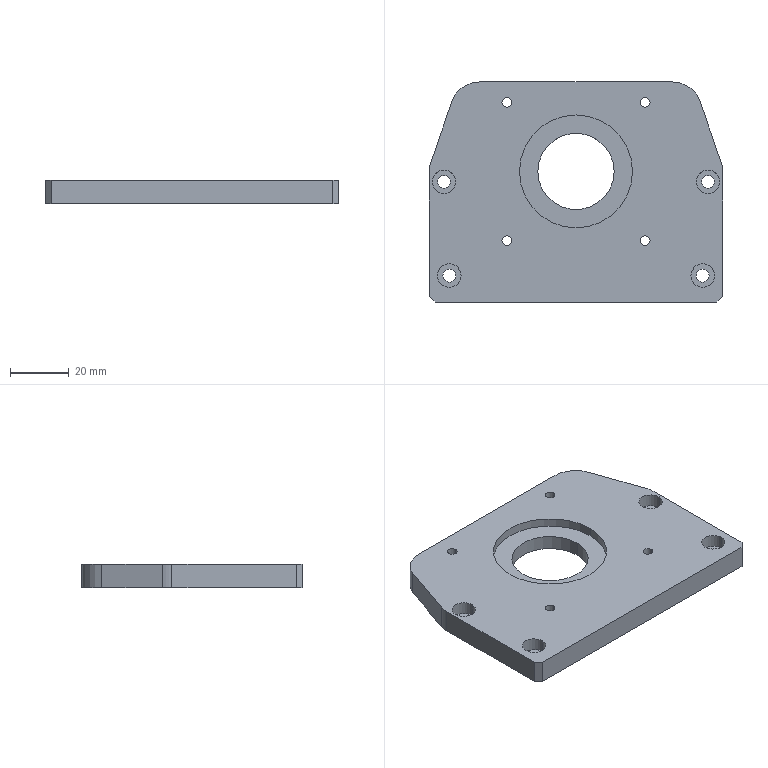Part | SolidWorks | features Cut 2, HoleWzd 2, Chamfer 1, Extrusion 1, Fillet 1, ICE 1 | 1 solid | 47 faces | box 100 x 75 x 8 mm | volume 49957 mm3 | cylinder 32 | plane 15 | commonest cylinder face diameters 3.3 x8 4.4 x8 8 x8 20 x4 26 x2 38.5 x2
STEP:
#1=CARTESIAN_POINT('',(-25.22,-16.57,0.));
#2=VERTEX_POINT('',#1);
#3=CARTESIAN_POINT('',(-21.92,-16.57,0.));
#4=VERTEX_POINT('',#3);
#5=CARTESIAN_POINT('',(-23.57,-16.57,0.));
#6=DIRECTION('',(0.,0.,1.));
#7=DIRECTION('',(1.,0.,0.));
#8=AXIS2_PLACEMENT_3D('',#5,#6,#7);
#9=CIRCLE('',#8,1.65);
#10=EDGE_CURVE('',#2,#4,#9,.T.);
#11=ORIENTED_EDGE('',*,*,#10,.F.);
#12=CARTESIAN_POINT('',(-25.22,-16.57,8.));
#13=VERTEX_POINT('',#12);
#14=CARTESIAN_POINT('',(-25.22,-16.57,8.));
#15=DIRECTION('',(0.,0.,1.));
#16=VECTOR('',#15,1000.);
#17=LINE('',#14,#16);
#18=EDGE_CURVE('',#2,#13,#17,.T.);
#19=ORIENTED_EDGE('',*,*,#18,.T.);
#20=CARTESIAN_POINT('',(-21.92,-16.57,8.));
#21=VERTEX_POINT('',#20);
#22=CARTESIAN_POINT('',(-23.57,-16.57,8.));
#23=DIRECTION('',(0.,0.,1.));
#24=DIRECTION('',(1.,0.,0.));
#25=AXIS2_PLACEMENT_3D('',#22,#23,#24);
#26=CIRCLE('',#25,1.65);
#27=EDGE_CURVE('',#13,#21,#26,.T.);
#28=ORIENTED_EDGE('',*,*,#27,.T.);
#29=CARTESIAN_POINT('',(-21.92,-16.57,8.));
#30=DIRECTION('',(0.,0.,1.));
#31=VECTOR('',#30,1000.);
#32=LINE('',#29,#31);
#33=EDGE_CURVE('',#4,#21,#32,.T.);
#34=ORIENTED_EDGE('',*,*,#33,.F.);
#35=EDGE_LOOP('',(#11,#19,#28,#34));
#36=FACE_OUTER_BOUND('',#35,.T.);
#37=CARTESIAN_POINT('',(-23.57,-16.57,8.));
#38=DIRECTION('',(0.,0.,1.));
#39=DIRECTION('',(1.,0.,0.));
#40=AXIS2_PLACEMENT_3D('',#37,#38,#39);
#41=CYLINDRICAL_SURFACE('',#40,1.65);
#42=ADVANCED_FACE('',(#36),#41,.F.);
#43=CARTESIAN_POINT('',(21.92,-16.57,0.));
#44=VERTEX_POINT('',#43);
#45=CARTESIAN_POINT('',(25.22,-16.57,0.));
#46=VERTEX_POINT('',#45);
#47=CARTESIAN_POINT('',(23.57,-16.57,0.));
#48=DIRECTION('',(0.,0.,1.));
#49=DIRECTION('',(1.,0.,0.));
#50=AXIS2_PLACEMENT_3D('',#47,#48,#49);
#51=CIRCLE('',#50,1.65);
#52=EDGE_CURVE('',#44,#46,#51,.T.);
#53=ORIENTED_EDGE('',*,*,#52,.F.);
#54=CARTESIAN_POINT('',(21.92,-16.57,8.));
#55=VERTEX_POINT('',#54);
#56=CARTESIAN_POINT('',(21.92,-16.57,8.));
#57=DIRECTION('',(0.,0.,1.));
#58=VECTOR('',#57,1000.);
#59=LINE('',#56,#58);
#60=EDGE_CURVE('',#44,#55,#59,.T.);
#61=ORIENTED_EDGE('',*,*,#60,.T.);
#62=CARTESIAN_POINT('',(25.22,-16.57,8.));
#63=VERTEX_POINT('',#62);
#64=CARTESIAN_POINT('',(23.57,-16.57,8.));
#65=DIRECTION('',(0.,0.,1.));
#66=DIRECTION('',(1.,0.,0.));
#67=AXIS2_PLACEMENT_3D('',#64,#65,#66);
#68=CIRCLE('',#67,1.65);
#69=EDGE_CURVE('',#55,#63,#68,.T.);
#70=ORIENTED_EDGE('',*,*,#69,.T.);
#71=CARTESIAN_POINT('',(25.22,-16.57,8.));
#72=DIRECTION('',(0.,0.,1.));
#73=VECTOR('',#72,1000.);
#74=LINE('',#71,#73);
#75=EDGE_CURVE('',#46,#63,#74,.T.);
#76=ORIENTED_EDGE('',*,*,#75,.F.);
#77=EDGE_LOOP('',(#53,#61,#70,#76));
#78=FACE_OUTER_BOUND('',#77,.T.);
#79=CARTESIAN_POINT('',(23.57,-16.57,8.));
#80=DIRECTION('',(0.,0.,1.));
#81=DIRECTION('',(1.,0.,0.));
#82=AXIS2_PLACEMENT_3D('',#79,#80,#81);
#83=CYLINDRICAL_SURFACE('',#82,1.65);
#84=ADVANCED_FACE('',(#78),#83,.F.);
#85=CARTESIAN_POINT('',(21.92,30.57,0.));
#86=VERTEX_POINT('',#85);
#87=CARTESIAN_POINT('',(25.22,30.57,0.));
#88=VERTEX_POINT('',#87);
#89=CARTESIAN_POINT('',(23.57,30.57,0.));
#90=DIRECTION('',(0.,0.,1.));
#91=DIRECTION('',(1.,0.,0.));
#92=AXIS2_PLACEMENT_3D('',#89,#90,#91);
#93=CIRCLE('',#92,1.65);
#94=EDGE_CURVE('',#86,#88,#93,.T.);
#95=ORIENTED_EDGE('',*,*,#94,.F.);
#96=CARTESIAN_POINT('',(21.92,30.57,8.));
#97=VERTEX_POINT('',#96);
#98=CARTESIAN_POINT('',(21.92,30.57,8.));
#99=DIRECTION('',(0.,0.,1.));
#100=VECTOR('',#99,1000.);
#101=LINE('',#98,#100);
#102=EDGE_CURVE('',#86,#97,#101,.T.);
#103=ORIENTED_EDGE('',*,*,#102,.T.);
#104=CARTESIAN_POINT('',(25.22,30.57,8.));
#105=VERTEX_POINT('',#104);
#106=CARTESIAN_POINT('',(23.57,30.57,8.));
#107=DIRECTION('',(0.,0.,1.));
#108=DIRECTION('',(1.,0.,0.));
#109=AXIS2_PLACEMENT_3D('',#106,#107,#108);
#110=CIRCLE('',#109,1.65);
#111=EDGE_CURVE('',#97,#105,#110,.T.);
#112=ORIENTED_EDGE('',*,*,#111,.T.);
#113=CARTESIAN_POINT('',(25.22,30.57,8.));
#114=DIRECTION('',(0.,0.,1.));
#115=VECTOR('',#114,1000.);
#116=LINE('',#113,#115);
#117=EDGE_CURVE('',#88,#105,#116,.T.);
#118=ORIENTED_EDGE('',*,*,#117,.F.);
#119=EDGE_LOOP('',(#95,#103,#112,#118));
#120=FACE_OUTER_BOUND('',#119,.T.);
#121=CARTESIAN_POINT('',(23.57,30.57,8.));
#122=DIRECTION('',(0.,0.,1.));
#123=DIRECTION('',(1.,0.,0.));
#124=AXIS2_PLACEMENT_3D('',#121,#122,#123);
#125=CYLINDRICAL_SURFACE('',#124,1.65);
#126=ADVANCED_FACE('',(#120),#125,.F.);
#127=CARTESIAN_POINT('',(-25.22,30.57,0.));
#128=VERTEX_POINT('',#127);
#129=CARTESIAN_POINT('',(-21.92,30.57,0.));
#130=VERTEX_POINT('',#129);
#131=CARTESIAN_POINT('',(-23.57,30.57,0.));
#132=DIRECTION('',(0.,0.,1.));
#133=DIRECTION('',(1.,0.,0.));
#134=AXIS2_PLACEMENT_3D('',#131,#132,#133);
#135=CIRCLE('',#134,1.65);
#136=EDGE_CURVE('',#128,#130,#135,.T.);
#137=ORIENTED_EDGE('',*,*,#136,.F.);
#138=CARTESIAN_POINT('',(-25.22,30.57,8.));
#139=VERTEX_POINT('',#138);
#140=CARTESIAN_POINT('',(-25.22,30.57,8.));
#141=DIRECTION('',(0.,0.,1.));
#142=VECTOR('',#141,1000.);
#143=LINE('',#140,#142);
#144=EDGE_CURVE('',#128,#139,#143,.T.);
#145=ORIENTED_EDGE('',*,*,#144,.T.);
#146=CARTESIAN_POINT('',(-21.92,30.57,8.));
#147=VERTEX_POINT('',#146);
#148=CARTESIAN_POINT('',(-23.57,30.57,8.));
#149=DIRECTION('',(0.,0.,1.));
#150=DIRECTION('',(1.,0.,0.));
#151=AXIS2_PLACEMENT_3D('',#148,#149,#150);
#152=CIRCLE('',#151,1.65);
#153=EDGE_CURVE('',#139,#147,#152,.T.);
#154=ORIENTED_EDGE('',*,*,#153,.T.);
#155=CARTESIAN_POINT('',(-21.92,30.57,8.));
#156=DIRECTION('',(0.,0.,1.));
#157=VECTOR('',#156,1000.);
#158=LINE('',#155,#157);
#159=EDGE_CURVE('',#130,#147,#158,.T.);
#160=ORIENTED_EDGE('',*,*,#159,.F.);
#161=EDGE_LOOP('',(#137,#145,#154,#160));
#162=FACE_OUTER_BOUND('',#161,.T.);
#163=CARTESIAN_POINT('',(-23.57,30.57,8.));
#164=DIRECTION('',(0.,0.,1.));
#165=DIRECTION('',(1.,0.,0.));
#166=AXIS2_PLACEMENT_3D('',#163,#164,#165);
#167=CYLINDRICAL_SURFACE('',#166,1.65);
#168=ADVANCED_FACE('',(#162),#167,.F.);
#169=CARTESIAN_POINT('',(-49.,3.5,3.5));
#170=VERTEX_POINT('',#169);
#171=CARTESIAN_POINT('',(-41.,3.5,3.5));
#172=VERTEX_POINT('',#171);
#173=CARTESIAN_POINT('',(-45.,3.5,3.5));
#174=DIRECTION('',(0.,0.,1.));
#175=DIRECTION('',(1.,0.,0.));
#176=AXIS2_PLACEMENT_3D('',#173,#174,#175);
#177=CIRCLE('',#176,4.);
#178=EDGE_CURVE('',#170,#172,#177,.T.);
#179=ORIENTED_EDGE('',*,*,#178,.F.);
#180=CARTESIAN_POINT('',(-49.,3.5,8.));
#181=VERTEX_POINT('',#180);
#182=CARTESIAN_POINT('',(-49.,3.5,8.));
#183=DIRECTION('',(0.,0.,1.));
#184=VECTOR('',#183,1000.);
#185=LINE('',#182,#184);
#186=EDGE_CURVE('',#170,#181,#185,.T.);
#187=ORIENTED_EDGE('',*,*,#186,.T.);
#188=CARTESIAN_POINT('',(-41.,3.5,8.));
#189=VERTEX_POINT('',#188);
#190=CARTESIAN_POINT('',(-45.,3.5,8.));
#191=DIRECTION('',(0.,0.,1.));
#192=DIRECTION('',(1.,0.,0.));
#193=AXIS2_PLACEMENT_3D('',#190,#191,#192);
#194=CIRCLE('',#193,4.);
#195=EDGE_CURVE('',#181,#189,#194,.T.);
#196=ORIENTED_EDGE('',*,*,#195,.T.);
#197=CARTESIAN_POINT('',(-41.,3.5,8.));
#198=DIRECTION('',(0.,0.,1.));
#199=VECTOR('',#198,1000.);
#200=LINE('',#197,#199);
#201=EDGE_CURVE('',#172,#189,#200,.T.);
#202=ORIENTED_EDGE('',*,*,#201,.F.);
#203=EDGE_LOOP('',(#179,#187,#196,#202));
#204=FACE_OUTER_BOUND('',#203,.T.);
#205=CARTESIAN_POINT('',(-45.,3.5,8.));
#206=DIRECTION('',(0.,0.,1.));
#207=DIRECTION('',(1.,0.,0.));
#208=AXIS2_PLACEMENT_3D('',#205,#206,#207);
#209=CYLINDRICAL_SURFACE('',#208,4.);
#210=ADVANCED_FACE('',(#204),#209,.F.);
#211=CARTESIAN_POINT('',(-47.2,3.5,0.));
#212=VERTEX_POINT('',#211);
#213=CARTESIAN_POINT('',(-42.8,3.5,0.));
#214=VERTEX_POINT('',#213);
#215=CARTESIAN_POINT('',(-45.,3.5,0.));
#216=DIRECTION('',(0.,0.,1.));
#217=DIRECTION('',(1.,0.,0.));
#218=AXIS2_PLACEMENT_3D('',#215,#216,#217);
#219=CIRCLE('',#218,2.2);
#220=EDGE_CURVE('',#212,#214,#219,.T.);
#221=ORIENTED_EDGE('',*,*,#220,.F.);
#222=CARTESIAN_POINT('',(-47.2,3.5,3.5));
#223=VERTEX_POINT('',#222);
#224=CARTESIAN_POINT('',(-47.2,3.5,8.));
#225=DIRECTION('',(0.,0.,1.));
#226=VECTOR('',#225,1000.);
#227=LINE('',#224,#226);
#228=EDGE_CURVE('',#212,#223,#227,.T.);
#229=ORIENTED_EDGE('',*,*,#228,.T.);
#230=CARTESIAN_POINT('',(-42.8,3.5,3.5));
#231=VERTEX_POINT('',#230);
#232=CARTESIAN_POINT('',(-45.,3.5,3.5));
#233=DIRECTION('',(0.,0.,1.));
#234=DIRECTION('',(1.,0.,0.));
#235=AXIS2_PLACEMENT_3D('',#232,#233,#234);
#236=CIRCLE('',#235,2.2);
#237=EDGE_CURVE('',#223,#231,#236,.T.);
#238=ORIENTED_EDGE('',*,*,#237,.T.);
#239=CARTESIAN_POINT('',(-42.8,3.5,8.));
#240=DIRECTION('',(0.,0.,1.));
#241=VECTOR('',#240,1000.);
#242=LINE('',#239,#241);
#243=EDGE_CURVE('',#214,#231,#242,.T.);
#244=ORIENTED_EDGE('',*,*,#243,.F.);
#245=EDGE_LOOP('',(#221,#229,#238,#244));
#246=FACE_OUTER_BOUND('',#245,.T.);
#247=CARTESIAN_POINT('',(-45.,3.5,8.));
#248=DIRECTION('',(0.,0.,1.));
#249=DIRECTION('',(1.,0.,0.));
#250=AXIS2_PLACEMENT_3D('',#247,#248,#249);
#251=CYLINDRICAL_SURFACE('',#250,2.2);
#252=ADVANCED_FACE('',(#246),#251,.F.);
#253=CARTESIAN_POINT('',(-47.15,-28.5,3.5));
#254=VERTEX_POINT('',#253);
#255=CARTESIAN_POINT('',(-39.15,-28.5,3.5));
#256=VERTEX_POINT('',#255);
#257=CARTESIAN_POINT('',(-43.15,-28.5,3.5));
#258=DIRECTION('',(0.,0.,1.));
#259=DIRECTION('',(1.,0.,0.));
#260=AXIS2_PLACEMENT_3D('',#257,#258,#259);
#261=CIRCLE('',#260,4.);
#262=EDGE_CURVE('',#254,#256,#261,.T.);
#263=ORIENTED_EDGE('',*,*,#262,.F.);
#264=CARTESIAN_POINT('',(-47.15,-28.5,8.));
#265=VERTEX_POINT('',#264);
#266=CARTESIAN_POINT('',(-47.15,-28.5,8.));
#267=DIRECTION('',(0.,0.,1.));
#268=VECTOR('',#267,1000.);
#269=LINE('',#266,#268);
#270=EDGE_CURVE('',#254,#265,#269,.T.);
#271=ORIENTED_EDGE('',*,*,#270,.T.);
#272=CARTESIAN_POINT('',(-39.15,-28.5,8.));
#273=VERTEX_POINT('',#272);
#274=CARTESIAN_POINT('',(-43.15,-28.5,8.));
#275=DIRECTION('',(0.,0.,1.));
#276=DIRECTION('',(1.,0.,0.));
#277=AXIS2_PLACEMENT_3D('',#274,#275,#276);
#278=CIRCLE('',#277,4.);
#279=EDGE_CURVE('',#265,#273,#278,.T.);
#280=ORIENTED_EDGE('',*,*,#279,.T.);
#281=CARTESIAN_POINT('',(-39.15,-28.5,8.));
#282=DIRECTION('',(0.,0.,1.));
#283=VECTOR('',#282,1000.);
#284=LINE('',#281,#283);
#285=EDGE_CURVE('',#256,#273,#284,.T.);
#286=ORIENTED_EDGE('',*,*,#285,.F.);
#287=EDGE_LOOP('',(#263,#271,#280,#286));
#288=FACE_OUTER_BOUND('',#287,.T.);
#289=CARTESIAN_POINT('',(-43.15,-28.5,8.));
#290=DIRECTION('',(0.,0.,1.));
#291=DIRECTION('',(1.,0.,0.));
#292=AXIS2_PLACEMENT_3D('',#289,#290,#291);
#293=CYLINDRICAL_SURFACE('',#292,4.);
#294=ADVANCED_FACE('',(#288),#293,.F.);
#295=CARTESIAN_POINT('',(-45.35,-28.5,0.));
#296=VERTEX_POINT('',#295);
#297=CARTESIAN_POINT('',(-40.95,-28.5,0.));
#298=VERTEX_POINT('',#297);
#299=CARTESIAN_POINT('',(-43.15,-28.5,0.));
#300=DIRECTION('',(0.,0.,1.));
#301=DIRECTION('',(1.,0.,0.));
#302=AXIS2_PLACEMENT_3D('',#299,#300,#301);
#303=CIRCLE('',#302,2.2);
#304=EDGE_CURVE('',#296,#298,#303,.T.);
#305=ORIENTED_EDGE('',*,*,#304,.F.);
#306=CARTESIAN_POINT('',(-45.35,-28.5,3.5));
#307=VERTEX_POINT('',#306);
#308=CARTESIAN_POINT('',(-45.35,-28.5,8.));
#309=DIRECTION('',(0.,0.,1.));
#310=VECTOR('',#309,1000.);
#311=LINE('',#308,#310);
#312=EDGE_CURVE('',#296,#307,#311,.T.);
#313=ORIENTED_EDGE('',*,*,#312,.T.);
#314=CARTESIAN_POINT('',(-40.95,-28.5,3.5));
#315=VERTEX_POINT('',#314);
#316=CARTESIAN_POINT('',(-43.15,-28.5,3.5));
#317=DIRECTION('',(0.,0.,1.));
#318=DIRECTION('',(1.,0.,0.));
#319=AXIS2_PLACEMENT_3D('',#316,#317,#318);
#320=CIRCLE('',#319,2.2);
#321=EDGE_CURVE('',#307,#315,#320,.T.);
#322=ORIENTED_EDGE('',*,*,#321,.T.);
#323=CARTESIAN_POINT('',(-40.95,-28.5,8.));
#324=DIRECTION('',(0.,0.,1.));
#325=VECTOR('',#324,1000.);
#326=LINE('',#323,#325);
#327=EDGE_CURVE('',#298,#315,#326,.T.);
#328=ORIENTED_EDGE('',*,*,#327,.F.);
#329=EDGE_LOOP('',(#305,#313,#322,#328));
#330=FACE_OUTER_BOUND('',#329,.T.);
#331=CARTESIAN_POINT('',(-43.15,-28.5,8.));
#332=DIRECTION('',(0.,0.,1.));
#333=DIRECTION('',(1.,0.,0.));
#334=AXIS2_PLACEMENT_3D('',#331,#332,#333);
#335=CYLINDRICAL_SURFACE('',#334,2.2);
#336=ADVANCED_FACE('',(#330),#335,.F.);
#337=CARTESIAN_POINT('',(39.15,-28.5,3.5));
#338=VERTEX_POINT('',#337);
#339=CARTESIAN_POINT('',(47.15,-28.5,3.5));
#340=VERTEX_POINT('',#339);
#341=CARTESIAN_POINT('',(43.15,-28.5,3.5));
#342=DIRECTION('',(0.,0.,1.));
#343=DIRECTION('',(1.,0.,0.));
#344=AXIS2_PLACEMENT_3D('',#341,#342,#343);
#345=CIRCLE('',#344,4.);
#346=EDGE_CURVE('',#338,#340,#345,.T.);
#347=ORIENTED_EDGE('',*,*,#346,.F.);
#348=CARTESIAN_POINT('',(39.15,-28.5,8.));
#349=VERTEX_POINT('',#348);
#350=CARTESIAN_POINT('',(39.15,-28.5,8.));
#351=DIRECTION('',(0.,0.,1.));
#352=VECTOR('',#351,1000.);
#353=LINE('',#350,#352);
#354=EDGE_CURVE('',#338,#349,#353,.T.);
#355=ORIENTED_EDGE('',*,*,#354,.T.);
#356=CARTESIAN_POINT('',(47.15,-28.5,8.));
#357=VERTEX_POINT('',#356);
#358=CARTESIAN_POINT('',(43.15,-28.5,8.));
#359=DIRECTION('',(0.,0.,1.));
#360=DIRECTION('',(1.,0.,0.));
#361=AXIS2_PLACEMENT_3D('',#358,#359,#360);
#362=CIRCLE('',#361,4.);
#363=EDGE_CURVE('',#349,#357,#362,.T.);
#364=ORIENTED_EDGE('',*,*,#363,.T.);
#365=CARTESIAN_POINT('',(47.15,-28.5,8.));
#366=DIRECTION('',(0.,0.,1.));
#367=VECTOR('',#366,1000.);
#368=LINE('',#365,#367);
#369=EDGE_CURVE('',#340,#357,#368,.T.);
#370=ORIENTED_EDGE('',*,*,#369,.F.);
#371=EDGE_LOOP('',(#347,#355,#364,#370));
#372=FACE_OUTER_BOUND('',#371,.T.);
#373=CARTESIAN_POINT('',(43.15,-28.5,8.));
#374=DIRECTION('',(0.,0.,1.));
#375=DIRECTION('',(1.,0.,0.));
#376=AXIS2_PLACEMENT_3D('',#373,#374,#375);
#377=CYLINDRICAL_SURFACE('',#376,4.);
#378=ADVANCED_FACE('',(#372),#377,.F.);
#379=CARTESIAN_POINT('',(40.95,-28.5,0.));
#380=VERTEX_POINT('',#379);
#381=CARTESIAN_POINT('',(45.35,-28.5,0.));
#382=VERTEX_POINT('',#381);
#383=CARTESIAN_POINT('',(43.15,-28.5,0.));
#384=DIRECTION('',(0.,0.,1.));
#385=DIRECTION('',(1.,0.,0.));
#386=AXIS2_PLACEMENT_3D('',#383,#384,#385);
#387=CIRCLE('',#386,2.2);
#388=EDGE_CURVE('',#380,#382,#387,.T.);
#389=ORIENTED_EDGE('',*,*,#388,.F.);
#390=CARTESIAN_POINT('',(40.95,-28.5,3.5));
#391=VERTEX_POINT('',#390);
#392=CARTESIAN_POINT('',(40.95,-28.5,8.));
#393=DIRECTION('',(0.,0.,1.));
#394=VECTOR('',#393,1000.);
#395=LINE('',#392,#394);
#396=EDGE_CURVE('',#380,#391,#395,.T.);
#397=ORIENTED_EDGE('',*,*,#396,.T.);
#398=CARTESIAN_POINT('',(45.35,-28.5,3.5));
#399=VERTEX_POINT('',#398);
#400=CARTESIAN_POINT('',(43.15,-28.5,3.5));
#401=DIRECTION('',(0.,0.,1.));
#402=DIRECTION('',(1.,0.,0.));
#403=AXIS2_PLACEMENT_3D('',#400,#401,#402);
#404=CIRCLE('',#403,2.2);
#405=EDGE_CURVE('',#391,#399,#404,.T.);
#406=ORIENTED_EDGE('',*,*,#405,.T.);
#407=CARTESIAN_POINT('',(45.35,-28.5,8.));
#408=DIRECTION('',(0.,0.,1.));
#409=VECTOR('',#408,1000.);
#410=LINE('',#407,#409);
#411=EDGE_CURVE('',#382,#399,#410,.T.);
#412=ORIENTED_EDGE('',*,*,#411,.F.);
#413=EDGE_LOOP('',(#389,#397,#406,#412));
#414=FACE_OUTER_BOUND('',#413,.T.);
#415=CARTESIAN_POINT('',(43.15,-28.5,8.));
#416=DIRECTION('',(0.,0.,1.));
#417=DIRECTION('',(1.,0.,0.));
#418=AXIS2_PLACEMENT_3D('',#415,#416,#417);
#419=CYLINDRICAL_SURFACE('',#418,2.2);
#420=ADVANCED_FACE('',(#414),#419,.F.);
#421=CARTESIAN_POINT('',(41.,3.5,3.5));
#422=VERTEX_POINT('',#421);
#423=CARTESIAN_POINT('',(49.,3.5,3.5));
#424=VERTEX_POINT('',#423);
#425=CARTESIAN_POINT('',(45.,3.5,3.5));
#426=DIRECTION('',(0.,0.,1.));
#427=DIRECTION('',(1.,0.,0.));
#428=AXIS2_PLACEMENT_3D('',#425,#426,#427);
#429=CIRCLE('',#428,4.);
#430=EDGE_CURVE('',#422,#424,#429,.T.);
#431=ORIENTED_EDGE('',*,*,#430,.F.);
#432=CARTESIAN_POINT('',(41.,3.5,8.));
#433=VERTEX_POINT('',#432);
#434=CARTESIAN_POINT('',(41.,3.5,8.));
#435=DIRECTION('',(0.,0.,1.));
#436=VECTOR('',#435,1000.);
#437=LINE('',#434,#436);
#438=EDGE_CURVE('',#422,#433,#437,.T.);
#439=ORIENTED_EDGE('',*,*,#438,.T.);
#440=CARTESIAN_POINT('',(49.,3.5,8.));
#441=VERTEX_POINT('',#440);
#442=CARTESIAN_POINT('',(45.,3.5,8.));
#443=DIRECTION('',(0.,0.,1.));
#444=DIRECTION('',(1.,0.,0.));
#445=AXIS2_PLACEMENT_3D('',#442,#443,#444);
#446=CIRCLE('',#445,4.);
#447=EDGE_CURVE('',#433,#441,#446,.T.);
#448=ORIENTED_EDGE('',*,*,#447,.T.);
#449=CARTESIAN_POINT('',(49.,3.5,8.));
#450=DIRECTION('',(0.,0.,1.));
#451=VECTOR('',#450,1000.);
#452=LINE('',#449,#451);
#453=EDGE_CURVE('',#424,#441,#452,.T.);
#454=ORIENTED_EDGE('',*,*,#453,.F.);
#455=EDGE_LOOP('',(#431,#439,#448,#454));
#456=FACE_OUTER_BOUND('',#455,.T.);
#457=CARTESIAN_POINT('',(45.,3.5,8.));
#458=DIRECTION('',(0.,0.,1.));
#459=DIRECTION('',(1.,0.,0.));
#460=AXIS2_PLACEMENT_3D('',#457,#458,#459);
#461=CYLINDRICAL_SURFACE('',#460,4.);
#462=ADVANCED_FACE('',(#456),#461,.F.);
#463=CARTESIAN_POINT('',(42.8,3.5,0.));
#464=VERTEX_POINT('',#463);
#465=CARTESIAN_POINT('',(47.2,3.5,0.));
#466=VERTEX_POINT('',#465);
#467=CARTESIAN_POINT('',(45.,3.5,0.));
#468=DIRECTION('',(0.,0.,1.));
#469=DIRECTION('',(1.,0.,0.));
#470=AXIS2_PLACEMENT_3D('',#467,#468,#469);
#471=CIRCLE('',#470,2.2);
#472=EDGE_CURVE('',#464,#466,#471,.T.);
#473=ORIENTED_EDGE('',*,*,#472,.F.);
#474=CARTESIAN_POINT('',(42.8,3.5,3.5));
#475=VERTEX_POINT('',#474);
#476=CARTESIAN_POINT('',(42.8,3.5,8.));
#477=DIRECTION('',(0.,0.,1.));
#478=VECTOR('',#477,1000.);
#479=LINE('',#476,#478);
#480=EDGE_CURVE('',#464,#475,#479,.T.);
#481=ORIENTED_EDGE('',*,*,#480,.T.);
#482=CARTESIAN_POINT('',(47.2,3.5,3.5));
#483=VERTEX_POINT('',#482);
#484=CARTESIAN_POINT('',(45.,3.5,3.5));
#485=DIRECTION('',(0.,0.,1.));
#486=DIRECTION('',(1.,0.,0.));
#487=AXIS2_PLACEMENT_3D('',#484,#485,#486);
#488=CIRCLE('',#487,2.2);
#489=EDGE_CURVE('',#475,#483,#488,.T.);
#490=ORIENTED_EDGE('',*,*,#489,.T.);
#491=CARTESIAN_POINT('',(47.2,3.5,8.));
#492=DIRECTION('',(0.,0.,1.));
#493=VECTOR('',#492,1000.);
#494=LINE('',#491,#493);
#495=EDGE_CURVE('',#466,#483,#494,.T.);
#496=ORIENTED_EDGE('',*,*,#495,.F.);
#497=EDGE_LOOP('',(#473,#481,#490,#496));
#498=FACE_OUTER_BOUND('',#497,.T.);
#499=CARTESIAN_POINT('',(45.,3.5,8.));
#500=DIRECTION('',(0.,0.,1.));
#501=DIRECTION('',(1.,0.,0.));
#502=AXIS2_PLACEMENT_3D('',#499,#500,#501);
#503=CYLINDRICAL_SURFACE('',#502,2.2);
#504=ADVANCED_FACE('',(#498),#503,.F.);
#505=CARTESIAN_POINT('',(-13.,7.,0.));
#506=VERTEX_POINT('',#505);
#507=CARTESIAN_POINT('',(13.,7.,0.));
#508=VERTEX_POINT('',#507);
#509=CARTESIAN_POINT('',(0.,7.,0.));
#510=DIRECTION('',(0.,0.,1.));
#511=DIRECTION('',(1.,0.,0.));
#512=AXIS2_PLACEMENT_3D('',#509,#510,#511);
#513=CIRCLE('',#512,13.);
#514=EDGE_CURVE('',#506,#508,#513,.T.);
#515=ORIENTED_EDGE('',*,*,#514,.F.);
#516=CARTESIAN_POINT('',(-13.,7.,5.));
#517=VERTEX_POINT('',#516);
#518=CARTESIAN_POINT('',(-13.,7.,0.));
#519=DIRECTION('',(0.,0.,1.));
#520=VECTOR('',#519,1000.);
#521=LINE('',#518,#520);
#522=EDGE_CURVE('',#506,#517,#521,.T.);
#523=ORIENTED_EDGE('',*,*,#522,.T.);
#524=CARTESIAN_POINT('',(13.,7.,5.));
#525=VERTEX_POINT('',#524);
#526=CARTESIAN_POINT('',(0.,7.,5.));
#527=DIRECTION('',(0.,0.,1.));
#528=DIRECTION('',(1.,0.,0.));
#529=AXIS2_PLACEMENT_3D('',#526,#527,#528);
#530=CIRCLE('',#529,13.);
#531=EDGE_CURVE('',#517,#525,#530,.T.);
#532=ORIENTED_EDGE('',*,*,#531,.T.);
#533=CARTESIAN_POINT('',(13.,7.,0.));
#534=DIRECTION('',(0.,0.,1.));
#535=VECTOR('',#534,1000.);
#536=LINE('',#533,#535);
#537=EDGE_CURVE('',#508,#525,#536,.T.);
#538=ORIENTED_EDGE('',*,*,#537,.F.);
#539=EDGE_LOOP('',(#515,#523,#532,#538));
#540=FACE_OUTER_BOUND('',#539,.T.);
#541=CARTESIAN_POINT('',(0.,7.,0.));
#542=DIRECTION('',(0.,0.,1.));
#543=DIRECTION('',(1.,0.,0.));
#544=AXIS2_PLACEMENT_3D('',#541,#542,#543);
#545=CYLINDRICAL_SURFACE('',#544,13.);
#546=ADVANCED_FACE('',(#540),#545,.F.);
#547=CARTESIAN_POINT('',(-19.25,7.,5.));
#548=VERTEX_POINT('',#547);
#549=CARTESIAN_POINT('',(19.25,7.,5.));
#550=VERTEX_POINT('',#549);
#551=CARTESIAN_POINT('',(0.,7.,5.));
#552=DIRECTION('',(0.,0.,1.));
#553=DIRECTION('',(1.,0.,0.));
#554=AXIS2_PLACEMENT_3D('',#551,#552,#553);
#555=CIRCLE('',#554,19.25);
#556=EDGE_CURVE('',#548,#550,#555,.T.);
#557=ORIENTED_EDGE('',*,*,#556,.F.);
#558=CARTESIAN_POINT('',(-19.25,7.,8.));
#559=VERTEX_POINT('',#558);
#560=CARTESIAN_POINT('',(-19.25,7.,5.));
#561=DIRECTION('',(0.,0.,1.));
#562=VECTOR('',#561,1000.);
#563=LINE('',#560,#562);
#564=EDGE_CURVE('',#548,#559,#563,.T.);
#565=ORIENTED_EDGE('',*,*,#564,.T.);
#566=CARTESIAN_POINT('',(19.25,7.,8.));
#567=VERTEX_POINT('',#566);
#568=CARTESIAN_POINT('',(0.,7.,8.));
#569=DIRECTION('',(0.,0.,1.));
#570=DIRECTION('',(1.,0.,0.));
#571=AXIS2_PLACEMENT_3D('',#568,#569,#570);
#572=CIRCLE('',#571,19.25);
#573=EDGE_CURVE('',#559,#567,#572,.T.);
#574=ORIENTED_EDGE('',*,*,#573,.T.);
#575=CARTESIAN_POINT('',(19.25,7.,5.));
#576=DIRECTION('',(0.,0.,1.));
#577=VECTOR('',#576,1000.);
#578=LINE('',#575,#577);
#579=EDGE_CURVE('',#550,#567,#578,.T.);
#580=ORIENTED_EDGE('',*,*,#579,.F.);
#581=EDGE_LOOP('',(#557,#565,#574,#580));
#582=FACE_OUTER_BOUND('',#581,.T.);
#583=CARTESIAN_POINT('',(0.,7.,5.));
#584=DIRECTION('',(0.,0.,1.));
#585=DIRECTION('',(1.,0.,0.));
#586=AXIS2_PLACEMENT_3D('',#583,#584,#585);
#587=CYLINDRICAL_SURFACE('',#586,19.25);
#588=ADVANCED_FACE('',(#582),#587,.F.);
#589=CARTESIAN_POINT('',(50.,-35.5,8.));
#590=VERTEX_POINT('',#589);
#591=CARTESIAN_POINT('',(50.,6.824,8.));
#592=VERTEX_POINT('',#591);
#593=CARTESIAN_POINT('',(50.,-37.5,8.));
#594=DIRECTION('',(0.,1.,0.));
#595=VECTOR('',#594,1000.);
#596=LINE('',#593,#595);
#597=EDGE_CURVE('',#590,#592,#596,.T.);
#598=ORIENTED_EDGE('',*,*,#597,.F.);
#599=CARTESIAN_POINT('',(50.,-35.5,0.));
#600=VERTEX_POINT('',#599);
#601=CARTESIAN_POINT('',(50.,-35.5,8.));
#602=DIRECTION('',(0.,0.,-1.));
#603=VECTOR('',#602,1000.);
#604=LINE('',#601,#603);
#605=EDGE_CURVE('',#590,#600,#604,.T.);
#606=ORIENTED_EDGE('',*,*,#605,.T.);
#607=CARTESIAN_POINT('',(50.,6.824,0.));
#608=VERTEX_POINT('',#607);
#609=CARTESIAN_POINT('',(50.,-37.5,0.));
#610=DIRECTION('',(0.,1.,0.));
#611=VECTOR('',#610,1000.);
#612=LINE('',#609,#611);
#613=EDGE_CURVE('',#600,#608,#612,.T.);
#614=ORIENTED_EDGE('',*,*,#613,.T.);
#615=CARTESIAN_POINT('',(50.,6.824,8.));
#616=DIRECTION('',(0.,0.,1.));
#617=VECTOR('',#616,1000.);
#618=LINE('',#615,#617);
#619=EDGE_CURVE('',#608,#592,#618,.T.);
#620=ORIENTED_EDGE('',*,*,#619,.T.);
#621=EDGE_LOOP('',(#598,#606,#614,#620));
#622=FACE_OUTER_BOUND('',#621,.T.);
#623=CARTESIAN_POINT('',(50.,-37.5,8.));
#624=DIRECTION('',(-1.,0.,0.));
#625=DIRECTION('',(0.,0.,1.));
#626=AXIS2_PLACEMENT_3D('',#623,#624,#625);
#627=PLANE('',#626);
#628=ADVANCED_FACE('',(#622),#627,.F.);
#629=CARTESIAN_POINT('',(32.87,37.5,0.));
#630=VERTEX_POINT('',#629);
#631=CARTESIAN_POINT('',(-32.87,37.5,0.));
#632=VERTEX_POINT('',#631);
#633=CARTESIAN_POINT('',(-50.,37.5,0.));
#634=DIRECTION('',(-1.,0.,0.));
#635=VECTOR('',#634,1000.);
#636=LINE('',#633,#635);
#637=EDGE_CURVE('',#630,#632,#636,.T.);
#638=ORIENTED_EDGE('',*,*,#637,.T.);
#639=CARTESIAN_POINT('',(-32.87,37.5,8.));
#640=VERTEX_POINT('',#639);
#641=CARTESIAN_POINT('',(-32.87,37.5,8.));
#642=DIRECTION('',(0.,0.,1.));
#643=VECTOR('',#642,1000.);
#644=LINE('',#641,#643);
#645=EDGE_CURVE('',#632,#640,#644,.T.);
#646=ORIENTED_EDGE('',*,*,#645,.T.);
#647=CARTESIAN_POINT('',(32.87,37.5,8.));
#648=VERTEX_POINT('',#647);
#649=CARTESIAN_POINT('',(-50.,37.5,8.));
#650=DIRECTION('',(-1.,0.,0.));
#651=VECTOR('',#650,1000.);
#652=LINE('',#649,#651);
#653=EDGE_CURVE('',#648,#640,#652,.T.);
#654=ORIENTED_EDGE('',*,*,#653,.F.);
#655=CARTESIAN_POINT('',(32.87,37.5,8.));
#656=DIRECTION('',(0.,0.,-1.));
#657=VECTOR('',#656,1000.);
#658=LINE('',#655,#657);
#659=EDGE_CURVE('',#648,#630,#658,.T.);
#660=ORIENTED_EDGE('',*,*,#659,.T.);
#661=EDGE_LOOP('',(#638,#646,#654,#660));
#662=FACE_OUTER_BOUND('',#661,.T.);
#663=CARTESIAN_POINT('',(-50.,37.5,8.));
#664=DIRECTION('',(0.,-1.,0.));
#665=DIRECTION('',(0.,0.,-1.));
#666=AXIS2_PLACEMENT_3D('',#663,#664,#665);
#667=PLANE('',#666);
#668=ADVANCED_FACE('',(#662),#667,.F.);
#669=CARTESIAN_POINT('',(-50.,6.824,0.));
#670=VERTEX_POINT('',#669);
#671=CARTESIAN_POINT('',(-50.,-35.5,0.));
#672=VERTEX_POINT('',#671);
#673=CARTESIAN_POINT('',(-50.,-37.5,0.));
#674=DIRECTION('',(0.,-1.,0.));
#675=VECTOR('',#674,1000.);
#676=LINE('',#673,#675);
#677=EDGE_CURVE('',#670,#672,#676,.T.);
#678=ORIENTED_EDGE('',*,*,#677,.T.);
#679=CARTESIAN_POINT('',(-50.,-35.5,8.));
#680=VERTEX_POINT('',#679);
#681=CARTESIAN_POINT('',(-50.,-35.5,8.));
#682=DIRECTION('',(0.,0.,1.));
#683=VECTOR('',#682,1000.);
#684=LINE('',#681,#683);
#685=EDGE_CURVE('',#672,#680,#684,.T.);
#686=ORIENTED_EDGE('',*,*,#685,.T.);
#687=CARTESIAN_POINT('',(-50.,6.824,8.));
#688=VERTEX_POINT('',#687);
#689=CARTESIAN_POINT('',(-50.,-37.5,8.));
#690=DIRECTION('',(0.,-1.,0.));
#691=VECTOR('',#690,1000.);
#692=LINE('',#689,#691);
#693=EDGE_CURVE('',#688,#680,#692,.T.);
#694=ORIENTED_EDGE('',*,*,#693,.F.);
#695=CARTESIAN_POINT('',(-50.,6.824,8.));
#696=DIRECTION('',(0.,0.,-1.));
#697=VECTOR('',#696,1000.);
#698=LINE('',#695,#697);
#699=EDGE_CURVE('',#688,#670,#698,.T.);
#700=ORIENTED_EDGE('',*,*,#699,.T.);
#701=EDGE_LOOP('',(#678,#686,#694,#700));
#702=FACE_OUTER_BOUND('',#701,.T.);
#703=CARTESIAN_POINT('',(-50.,-37.5,8.));
#704=DIRECTION('',(1.,0.,0.));
#705=DIRECTION('',(0.,0.,-1.));
#706=AXIS2_PLACEMENT_3D('',#703,#704,#705);
#707=PLANE('',#706);
#708=ADVANCED_FACE('',(#702),#707,.F.);
#709=CARTESIAN_POINT('',(-48.,-37.5,8.));
#710=VERTEX_POINT('',#709);
#711=CARTESIAN_POINT('',(48.,-37.5,8.));
#712=VERTEX_POINT('',#711);
#713=CARTESIAN_POINT('',(-50.,-37.5,8.));
#714=DIRECTION('',(1.,0.,0.));
#715=VECTOR('',#714,1000.);
#716=LINE('',#713,#715);
#717=EDGE_CURVE('',#710,#712,#716,.T.);
#718=ORIENTED_EDGE('',*,*,#717,.F.);
#719=CARTESIAN_POINT('',(-48.,-37.5,0.));
#720=VERTEX_POINT('',#719);
#721=CARTESIAN_POINT('',(-48.,-37.5,8.));
#722=DIRECTION('',(0.,0.,-1.));
#723=VECTOR('',#722,1000.);
#724=LINE('',#721,#723);
#725=EDGE_CURVE('',#710,#720,#724,.T.);
#726=ORIENTED_EDGE('',*,*,#725,.T.);
#727=CARTESIAN_POINT('',(48.,-37.5,0.));
#728=VERTEX_POINT('',#727);
#729=CARTESIAN_POINT('',(-50.,-37.5,0.));
#730=DIRECTION('',(1.,0.,0.));
#731=VECTOR('',#730,1000.);
#732=LINE('',#729,#731);
#733=EDGE_CURVE('',#720,#728,#732,.T.);
#734=ORIENTED_EDGE('',*,*,#733,.T.);
#735=CARTESIAN_POINT('',(48.,-37.5,8.));
#736=DIRECTION('',(0.,0.,1.));
#737=VECTOR('',#736,1000.);
#738=LINE('',#735,#737);
#739=EDGE_CURVE('',#728,#712,#738,.T.);
#740=ORIENTED_EDGE('',*,*,#739,.T.);
#741=EDGE_LOOP('',(#718,#726,#734,#740));
#742=FACE_OUTER_BOUND('',#741,.T.);
#743=CARTESIAN_POINT('',(-50.,-37.5,8.));
#744=DIRECTION('',(0.,1.,0.));
#745=DIRECTION('',(0.,0.,1.));
#746=AXIS2_PLACEMENT_3D('',#743,#744,#745);
#747=PLANE('',#746);
#748=ADVANCED_FACE('',(#742),#747,.F.);
#749=CARTESIAN_POINT('',(-23.57,-16.57,8.));
#750=DIRECTION('',(0.,0.,1.));
#751=DIRECTION('',(1.,0.,0.));
#752=AXIS2_PLACEMENT_3D('',#749,#750,#751);
#753=CIRCLE('',#752,1.65);
#754=EDGE_CURVE('',#21,#13,#753,.T.);
#755=ORIENTED_EDGE('',*,*,#754,.F.);
#756=ORIENTED_EDGE('',*,*,#27,.F.);
#757=EDGE_LOOP('',(#755,#756));
#758=FACE_BOUND('',#757,.T.);
#759=CARTESIAN_POINT('',(23.57,-16.57,8.));
#760=DIRECTION('',(0.,0.,1.));
#761=DIRECTION('',(1.,0.,0.));
#762=AXIS2_PLACEMENT_3D('',#759,#760,#761);
#763=CIRCLE('',#762,1.65);
#764=EDGE_CURVE('',#63,#55,#763,.T.);
#765=ORIENTED_EDGE('',*,*,#764,.F.);
#766=ORIENTED_EDGE('',*,*,#69,.F.);
#767=EDGE_LOOP('',(#765,#766));
#768=FACE_BOUND('',#767,.T.);
#769=CARTESIAN_POINT('',(23.57,30.57,8.));
#770=DIRECTION('',(0.,0.,1.));
#771=DIRECTION('',(1.,0.,0.));
#772=AXIS2_PLACEMENT_3D('',#769,#770,#771);
#773=CIRCLE('',#772,1.65);
#774=EDGE_CURVE('',#105,#97,#773,.T.);
#775=ORIENTED_EDGE('',*,*,#774,.F.);
#776=ORIENTED_EDGE('',*,*,#111,.F.);
#777=EDGE_LOOP('',(#775,#776));
#778=FACE_BOUND('',#777,.T.);
#779=CARTESIAN_POINT('',(-23.57,30.57,8.));
#780=DIRECTION('',(0.,0.,1.));
#781=DIRECTION('',(1.,0.,0.));
#782=AXIS2_PLACEMENT_3D('',#779,#780,#781);
#783=CIRCLE('',#782,1.65);
#784=EDGE_CURVE('',#147,#139,#783,.T.);
#785=ORIENTED_EDGE('',*,*,#784,.F.);
#786=ORIENTED_EDGE('',*,*,#153,.F.);
#787=EDGE_LOOP('',(#785,#786));
#788=FACE_BOUND('',#787,.T.);
#789=CARTESIAN_POINT('',(-45.,3.5,8.));
#790=DIRECTION('',(0.,0.,1.));
#791=DIRECTION('',(1.,0.,0.));
#792=AXIS2_PLACEMENT_3D('',#789,#790,#791);
#793=CIRCLE('',#792,4.);
#794=EDGE_CURVE('',#189,#181,#793,.T.);
#795=ORIENTED_EDGE('',*,*,#794,.F.);
#796=ORIENTED_EDGE('',*,*,#195,.F.);
#797=EDGE_LOOP('',(#795,#796));
#798=FACE_BOUND('',#797,.T.);
#799=CARTESIAN_POINT('',(-43.15,-28.5,8.));
#800=DIRECTION('',(0.,0.,1.));
#801=DIRECTION('',(1.,0.,0.));
#802=AXIS2_PLACEMENT_3D('',#799,#800,#801);
#803=CIRCLE('',#802,4.);
#804=EDGE_CURVE('',#273,#265,#803,.T.);
#805=ORIENTED_EDGE('',*,*,#804,.F.);
#806=ORIENTED_EDGE('',*,*,#279,.F.);
#807=EDGE_LOOP('',(#805,#806));
#808=FACE_BOUND('',#807,.T.);
#809=CARTESIAN_POINT('',(43.15,-28.5,8.));
#810=DIRECTION('',(0.,0.,1.));
#811=DIRECTION('',(1.,0.,0.));
#812=AXIS2_PLACEMENT_3D('',#809,#810,#811);
#813=CIRCLE('',#812,4.);
#814=EDGE_CURVE('',#357,#349,#813,.T.);
#815=ORIENTED_EDGE('',*,*,#814,.F.);
#816=ORIENTED_EDGE('',*,*,#363,.F.);
#817=EDGE_LOOP('',(#815,#816));
#818=FACE_BOUND('',#817,.T.);
#819=CARTESIAN_POINT('',(45.,3.5,8.));
#820=DIRECTION('',(0.,0.,1.));
#821=DIRECTION('',(1.,0.,0.));
#822=AXIS2_PLACEMENT_3D('',#819,#820,#821);
#823=CIRCLE('',#822,4.);
#824=EDGE_CURVE('',#441,#433,#823,.T.);
#825=ORIENTED_EDGE('',*,*,#824,.F.);
#826=ORIENTED_EDGE('',*,*,#447,.F.);
#827=EDGE_LOOP('',(#825,#826));
#828=FACE_BOUND('',#827,.T.);
#829=CARTESIAN_POINT('',(0.,7.,8.));
#830=DIRECTION('',(0.,0.,1.));
#831=DIRECTION('',(1.,0.,0.));
#832=AXIS2_PLACEMENT_3D('',#829,#830,#831);
#833=CIRCLE('',#832,19.25);
#834=EDGE_CURVE('',#567,#559,#833,.T.);
#835=ORIENTED_EDGE('',*,*,#834,.F.);
#836=ORIENTED_EDGE('',*,*,#573,.F.);
#837=EDGE_LOOP('',(#835,#836));
#838=FACE_BOUND('',#837,.T.);
#839=ORIENTED_EDGE('',*,*,#693,.T.);
#840=CARTESIAN_POINT('',(-48.,-37.5,8.));
#841=DIRECTION('',(0.7071,-0.7071,0.));
#842=VECTOR('',#841,1000.);
#843=LINE('',#840,#842);
#844=EDGE_CURVE('',#680,#710,#843,.T.);
#845=ORIENTED_EDGE('',*,*,#844,.T.);
#846=ORIENTED_EDGE('',*,*,#717,.T.);
#847=CARTESIAN_POINT('',(50.,-35.5,8.));
#848=DIRECTION('',(0.7071,0.7071,0.));
#849=VECTOR('',#848,1000.);
#850=LINE('',#847,#849);
#851=EDGE_CURVE('',#712,#590,#850,.T.);
#852=ORIENTED_EDGE('',*,*,#851,.T.);
#853=ORIENTED_EDGE('',*,*,#597,.T.);
#854=CARTESIAN_POINT('',(49.454,10.084,8.));
#855=VERTEX_POINT('',#854);
#856=CARTESIAN_POINT('',(40.,6.824,8.));
#857=DIRECTION('',(0.,0.,1.));
#858=DIRECTION('',(-1.,0.,0.));
#859=AXIS2_PLACEMENT_3D('',#856,#857,#858);
#860=CIRCLE('',#859,10.);
#861=EDGE_CURVE('',#592,#855,#860,.T.);
#862=ORIENTED_EDGE('',*,*,#861,.T.);
#863=CARTESIAN_POINT('',(42.324,30.76,8.));
#864=VERTEX_POINT('',#863);
#865=CARTESIAN_POINT('',(47.306,16.312,8.));
#866=DIRECTION('',(-0.326,0.9454,0.));
#867=VECTOR('',#866,1000.);
#868=LINE('',#865,#867);
#869=EDGE_CURVE('',#855,#864,#868,.T.);
#870=ORIENTED_EDGE('',*,*,#869,.T.);
#871=CARTESIAN_POINT('',(32.87,27.5,8.));
#872=DIRECTION('',(0.,0.,1.));
#873=DIRECTION('',(-1.,0.,0.));
#874=AXIS2_PLACEMENT_3D('',#871,#872,#873);
#875=CIRCLE('',#874,10.);
#876=EDGE_CURVE('',#864,#648,#875,.T.);
#877=ORIENTED_EDGE('',*,*,#876,.T.);
#878=ORIENTED_EDGE('',*,*,#653,.T.);
#879=CARTESIAN_POINT('',(-42.324,30.76,8.));
#880=VERTEX_POINT('',#879);
#881=CARTESIAN_POINT('',(-32.87,27.5,8.));
#882=DIRECTION('',(0.,0.,1.));
#883=DIRECTION('',(-1.,0.,0.));
#884=AXIS2_PLACEMENT_3D('',#881,#882,#883);
#885=CIRCLE('',#884,10.);
#886=EDGE_CURVE('',#640,#880,#885,.T.);
#887=ORIENTED_EDGE('',*,*,#886,.T.);
#888=CARTESIAN_POINT('',(-49.454,10.084,8.));
#889=VERTEX_POINT('',#888);
#890=CARTESIAN_POINT('',(-47.306,16.312,8.));
#891=DIRECTION('',(-0.326,-0.9454,0.));
#892=VECTOR('',#891,1000.);
#893=LINE('',#890,#892);
#894=EDGE_CURVE('',#880,#889,#893,.T.);
#895=ORIENTED_EDGE('',*,*,#894,.T.);
#896=CARTESIAN_POINT('',(-40.,6.824,8.));
#897=DIRECTION('',(0.,0.,1.));
#898=DIRECTION('',(-1.,0.,0.));
#899=AXIS2_PLACEMENT_3D('',#896,#897,#898);
#900=CIRCLE('',#899,10.);
#901=EDGE_CURVE('',#889,#688,#900,.T.);
#902=ORIENTED_EDGE('',*,*,#901,.T.);
#903=EDGE_LOOP('',(#839,#845,#846,#852,#853,#862,#870,#877,#878,#887,#895,#902));
#904=FACE_OUTER_BOUND('',#903,.T.);
#905=CARTESIAN_POINT('',(0.,0.,8.));
#906=DIRECTION('',(0.,0.,-1.));
#907=DIRECTION('',(-1.,0.,0.));
#908=AXIS2_PLACEMENT_3D('',#905,#906,#907);
#909=PLANE('',#908);
#910=ADVANCED_FACE('',(#758,#768,#778,#788,#798,#808,#818,#828,#838,#904),#909,.F.);
#911=CARTESIAN_POINT('',(-23.57,-16.57,0.));
#912=DIRECTION('',(0.,0.,1.));
#913=DIRECTION('',(1.,0.,0.));
#914=AXIS2_PLACEMENT_3D('',#911,#912,#913);
#915=CIRCLE('',#914,1.65);
#916=EDGE_CURVE('',#4,#2,#915,.T.);
#917=ORIENTED_EDGE('',*,*,#916,.T.);
#918=ORIENTED_EDGE('',*,*,#10,.T.);
#919=EDGE_LOOP('',(#917,#918));
#920=FACE_BOUND('',#919,.T.);
#921=CARTESIAN_POINT('',(23.57,-16.57,0.));
#922=DIRECTION('',(0.,0.,1.));
#923=DIRECTION('',(1.,0.,0.));
#924=AXIS2_PLACEMENT_3D('',#921,#922,#923);
#925=CIRCLE('',#924,1.65);
#926=EDGE_CURVE('',#46,#44,#925,.T.);
#927=ORIENTED_EDGE('',*,*,#926,.T.);
#928=ORIENTED_EDGE('',*,*,#52,.T.);
#929=EDGE_LOOP('',(#927,#928));
#930=FACE_BOUND('',#929,.T.);
#931=CARTESIAN_POINT('',(23.57,30.57,0.));
#932=DIRECTION('',(0.,0.,1.));
#933=DIRECTION('',(1.,0.,0.));
#934=AXIS2_PLACEMENT_3D('',#931,#932,#933);
#935=CIRCLE('',#934,1.65);
#936=EDGE_CURVE('',#88,#86,#935,.T.);
#937=ORIENTED_EDGE('',*,*,#936,.T.);
#938=ORIENTED_EDGE('',*,*,#94,.T.);
#939=EDGE_LOOP('',(#937,#938));
#940=FACE_BOUND('',#939,.T.);
#941=CARTESIAN_POINT('',(-23.57,30.57,0.));
#942=DIRECTION('',(0.,0.,1.));
#943=DIRECTION('',(1.,0.,0.));
#944=AXIS2_PLACEMENT_3D('',#941,#942,#943);
#945=CIRCLE('',#944,1.65);
#946=EDGE_CURVE('',#130,#128,#945,.T.);
#947=ORIENTED_EDGE('',*,*,#946,.T.);
#948=ORIENTED_EDGE('',*,*,#136,.T.);
#949=EDGE_LOOP('',(#947,#948));
#950=FACE_BOUND('',#949,.T.);
#951=CARTESIAN_POINT('',(-45.,3.5,0.));
#952=DIRECTION('',(0.,0.,1.));
#953=DIRECTION('',(1.,0.,0.));
#954=AXIS2_PLACEMENT_3D('',#951,#952,#953);
#955=CIRCLE('',#954,2.2);
#956=EDGE_CURVE('',#214,#212,#955,.T.);
#957=ORIENTED_EDGE('',*,*,#956,.T.);
#958=ORIENTED_EDGE('',*,*,#220,.T.);
#959=EDGE_LOOP('',(#957,#958));
#960=FACE_BOUND('',#959,.T.);
#961=CARTESIAN_POINT('',(-43.15,-28.5,0.));
#962=DIRECTION('',(0.,0.,1.));
#963=DIRECTION('',(1.,0.,0.));
#964=AXIS2_PLACEMENT_3D('',#961,#962,#963);
#965=CIRCLE('',#964,2.2);
#966=EDGE_CURVE('',#298,#296,#965,.T.);
#967=ORIENTED_EDGE('',*,*,#966,.T.);
#968=ORIENTED_EDGE('',*,*,#304,.T.);
#969=EDGE_LOOP('',(#967,#968));
#970=FACE_BOUND('',#969,.T.);
#971=CARTESIAN_POINT('',(43.15,-28.5,0.));
#972=DIRECTION('',(0.,0.,1.));
#973=DIRECTION('',(1.,0.,0.));
#974=AXIS2_PLACEMENT_3D('',#971,#972,#973);
#975=CIRCLE('',#974,2.2);
#976=EDGE_CURVE('',#382,#380,#975,.T.);
#977=ORIENTED_EDGE('',*,*,#976,.T.);
#978=ORIENTED_EDGE('',*,*,#388,.T.);
#979=EDGE_LOOP('',(#977,#978));
#980=FACE_BOUND('',#979,.T.);
#981=CARTESIAN_POINT('',(45.,3.5,0.));
#982=DIRECTION('',(0.,0.,1.));
#983=DIRECTION('',(1.,0.,0.));
#984=AXIS2_PLACEMENT_3D('',#981,#982,#983);
#985=CIRCLE('',#984,2.2);
#986=EDGE_CURVE('',#466,#464,#985,.T.);
#987=ORIENTED_EDGE('',*,*,#986,.T.);
#988=ORIENTED_EDGE('',*,*,#472,.T.);
#989=EDGE_LOOP('',(#987,#988));
#990=FACE_BOUND('',#989,.T.);
#991=CARTESIAN_POINT('',(0.,7.,0.));
#992=DIRECTION('',(0.,0.,1.));
#993=DIRECTION('',(1.,0.,0.));
#994=AXIS2_PLACEMENT_3D('',#991,#992,#993);
#995=CIRCLE('',#994,13.);
#996=EDGE_CURVE('',#508,#506,#995,.T.);
#997=ORIENTED_EDGE('',*,*,#996,.T.);
#998=ORIENTED_EDGE('',*,*,#514,.T.);
#999=EDGE_LOOP('',(#997,#998));
#1000=FACE_BOUND('',#999,.T.);
#1001=ORIENTED_EDGE('',*,*,#733,.F.);
#1002=CARTESIAN_POINT('',(-42.75,-42.75,0.));
#1003=DIRECTION('',(-0.7071,0.7071,0.));
#1004=VECTOR('',#1003,1000.);
#1005=LINE('',#1002,#1004);
#1006=EDGE_CURVE('',#720,#672,#1005,.T.);
#1007=ORIENTED_EDGE('',*,*,#1006,.T.);
#1008=ORIENTED_EDGE('',*,*,#677,.F.);
#1009=CARTESIAN_POINT('',(-49.454,10.084,0.));
#1010=VERTEX_POINT('',#1009);
#1011=CARTESIAN_POINT('',(-40.,6.824,0.));
#1012=DIRECTION('',(0.,0.,-1.));
#1013=DIRECTION('',(-1.,0.,0.));
#1014=AXIS2_PLACEMENT_3D('',#1011,#1012,#1013);
#1015=CIRCLE('',#1014,10.);
#1016=EDGE_CURVE('',#670,#1010,#1015,.T.);
#1017=ORIENTED_EDGE('',*,*,#1016,.T.);
#1018=CARTESIAN_POINT('',(-42.324,30.76,0.));
#1019=VERTEX_POINT('',#1018);
#1020=CARTESIAN_POINT('',(-50.,8.5,0.));
#1021=DIRECTION('',(-0.326,-0.9454,0.));
#1022=VECTOR('',#1021,1000.);
#1023=LINE('',#1020,#1022);
#1024=EDGE_CURVE('',#1019,#1010,#1023,.T.);
#1025=ORIENTED_EDGE('',*,*,#1024,.F.);
#1026=CARTESIAN_POINT('',(-32.87,27.5,0.));
#1027=DIRECTION('',(0.,0.,-1.));
#1028=DIRECTION('',(-1.,0.,0.));
#1029=AXIS2_PLACEMENT_3D('',#1026,#1027,#1028);
#1030=CIRCLE('',#1029,10.);
#1031=EDGE_CURVE('',#1019,#632,#1030,.T.);
#1032=ORIENTED_EDGE('',*,*,#1031,.T.);
#1033=ORIENTED_EDGE('',*,*,#637,.F.);
#1034=CARTESIAN_POINT('',(42.324,30.76,0.));
#1035=VERTEX_POINT('',#1034);
#1036=CARTESIAN_POINT('',(32.87,27.5,0.));
#1037=DIRECTION('',(0.,0.,-1.));
#1038=DIRECTION('',(-1.,0.,0.));
#1039=AXIS2_PLACEMENT_3D('',#1036,#1037,#1038);
#1040=CIRCLE('',#1039,10.);
#1041=EDGE_CURVE('',#630,#1035,#1040,.T.);
#1042=ORIENTED_EDGE('',*,*,#1041,.T.);
#1043=CARTESIAN_POINT('',(49.454,10.084,0.));
#1044=VERTEX_POINT('',#1043);
#1045=CARTESIAN_POINT('',(50.,8.5,0.));
#1046=DIRECTION('',(-0.326,0.9454,0.));
#1047=VECTOR('',#1046,1000.);
#1048=LINE('',#1045,#1047);
#1049=EDGE_CURVE('',#1044,#1035,#1048,.T.);
#1050=ORIENTED_EDGE('',*,*,#1049,.F.);
#1051=CARTESIAN_POINT('',(40.,6.824,0.));
#1052=DIRECTION('',(0.,0.,-1.));
#1053=DIRECTION('',(-1.,0.,0.));
#1054=AXIS2_PLACEMENT_3D('',#1051,#1052,#1053);
#1055=CIRCLE('',#1054,10.);
#1056=EDGE_CURVE('',#1044,#608,#1055,.T.);
#1057=ORIENTED_EDGE('',*,*,#1056,.T.);
#1058=ORIENTED_EDGE('',*,*,#613,.F.);
#1059=CARTESIAN_POINT('',(42.75,-42.75,0.));
#1060=DIRECTION('',(-0.7071,-0.7071,0.));
#1061=VECTOR('',#1060,1000.);
#1062=LINE('',#1059,#1061);
#1063=EDGE_CURVE('',#600,#728,#1062,.T.);
#1064=ORIENTED_EDGE('',*,*,#1063,.T.);
#1065=EDGE_LOOP('',(#1001,#1007,#1008,#1017,#1025,#1032,#1033,#1042,#1050,#1057,#1058,#1064));
#1066=FACE_OUTER_BOUND('',#1065,.T.);
#1067=CARTESIAN_POINT('',(0.,0.,0.));
#1068=DIRECTION('',(0.,0.,-1.));
#1069=DIRECTION('',(-1.,0.,0.));
#1070=AXIS2_PLACEMENT_3D('',#1067,#1068,#1069);
#1071=PLANE('',#1070);
#1072=ADVANCED_FACE('',(#920,#930,#940,#950,#960,#970,#980,#990,#1000,#1066),#1071,.T.);
#1073=ORIENTED_EDGE('',*,*,#1049,.T.);
#1074=CARTESIAN_POINT('',(42.324,30.76,10.));
#1075=DIRECTION('',(0.,0.,1.));
#1076=VECTOR('',#1075,1000.);
#1077=LINE('',#1074,#1076);
#1078=EDGE_CURVE('',#1035,#864,#1077,.T.);
#1079=ORIENTED_EDGE('',*,*,#1078,.T.);
#1080=ORIENTED_EDGE('',*,*,#869,.F.);
#1081=CARTESIAN_POINT('',(49.454,10.084,10.));
#1082=DIRECTION('',(0.,0.,-1.));
#1083=VECTOR('',#1082,1000.);
#1084=LINE('',#1081,#1083);
#1085=EDGE_CURVE('',#855,#1044,#1084,.T.);
#1086=ORIENTED_EDGE('',*,*,#1085,.T.);
#1087=EDGE_LOOP('',(#1073,#1079,#1080,#1086));
#1088=FACE_OUTER_BOUND('',#1087,.T.);
#1089=CARTESIAN_POINT('',(50.,8.5,10.));
#1090=DIRECTION('',(-0.9454,-0.326,0.));
#1091=DIRECTION('',(0.326,-0.9454,0.));
#1092=AXIS2_PLACEMENT_3D('',#1089,#1090,#1091);
#1093=PLANE('',#1092);
#1094=ADVANCED_FACE('',(#1088),#1093,.F.);
#1095=ORIENTED_EDGE('',*,*,#1024,.T.);
#1096=CARTESIAN_POINT('',(-49.454,10.084,10.));
#1097=DIRECTION('',(0.,0.,1.));
#1098=VECTOR('',#1097,1000.);
#1099=LINE('',#1096,#1098);
#1100=EDGE_CURVE('',#1010,#889,#1099,.T.);
#1101=ORIENTED_EDGE('',*,*,#1100,.T.);
#1102=ORIENTED_EDGE('',*,*,#894,.F.);
#1103=CARTESIAN_POINT('',(-42.324,30.76,10.));
#1104=DIRECTION('',(0.,0.,-1.));
#1105=VECTOR('',#1104,1000.);
#1106=LINE('',#1103,#1105);
#1107=EDGE_CURVE('',#880,#1019,#1106,.T.);
#1108=ORIENTED_EDGE('',*,*,#1107,.T.);
#1109=EDGE_LOOP('',(#1095,#1101,#1102,#1108));
#1110=FACE_OUTER_BOUND('',#1109,.T.);
#1111=CARTESIAN_POINT('',(-50.,8.5,10.));
#1112=DIRECTION('',(0.9454,-0.326,0.));
#1113=DIRECTION('',(0.326,0.9454,0.));
#1114=AXIS2_PLACEMENT_3D('',#1111,#1112,#1113);
#1115=PLANE('',#1114);
#1116=ADVANCED_FACE('',(#1110),#1115,.F.);
#1117=ORIENTED_EDGE('',*,*,#901,.F.);
#1118=ORIENTED_EDGE('',*,*,#1100,.F.);
#1119=ORIENTED_EDGE('',*,*,#1016,.F.);
#1120=ORIENTED_EDGE('',*,*,#699,.F.);
#1121=EDGE_LOOP('',(#1117,#1118,#1119,#1120));
#1122=FACE_OUTER_BOUND('',#1121,.T.);
#1123=CARTESIAN_POINT('',(-40.,6.824,8.));
#1124=DIRECTION('',(0.,0.,-1.));
#1125=DIRECTION('',(-1.,0.,0.));
#1126=AXIS2_PLACEMENT_3D('',#1123,#1124,#1125);
#1127=CYLINDRICAL_SURFACE('',#1126,10.);
#1128=ADVANCED_FACE('',(#1122),#1127,.T.);
#1129=ORIENTED_EDGE('',*,*,#886,.F.);
#1130=ORIENTED_EDGE('',*,*,#645,.F.);
#1131=ORIENTED_EDGE('',*,*,#1031,.F.);
#1132=ORIENTED_EDGE('',*,*,#1107,.F.);
#1133=EDGE_LOOP('',(#1129,#1130,#1131,#1132));
#1134=FACE_OUTER_BOUND('',#1133,.T.);
#1135=CARTESIAN_POINT('',(-32.87,27.5,10.));
#1136=DIRECTION('',(0.,0.,-1.));
#1137=DIRECTION('',(-1.,0.,0.));
#1138=AXIS2_PLACEMENT_3D('',#1135,#1136,#1137);
#1139=CYLINDRICAL_SURFACE('',#1138,10.);
#1140=ADVANCED_FACE('',(#1134),#1139,.T.);
#1141=ORIENTED_EDGE('',*,*,#876,.F.);
#1142=ORIENTED_EDGE('',*,*,#1078,.F.);
#1143=ORIENTED_EDGE('',*,*,#1041,.F.);
#1144=ORIENTED_EDGE('',*,*,#659,.F.);
#1145=EDGE_LOOP('',(#1141,#1142,#1143,#1144));
#1146=FACE_OUTER_BOUND('',#1145,.T.);
#1147=CARTESIAN_POINT('',(32.87,27.5,8.));
#1148=DIRECTION('',(0.,0.,-1.));
#1149=DIRECTION('',(-1.,0.,0.));
#1150=AXIS2_PLACEMENT_3D('',#1147,#1148,#1149);
#1151=CYLINDRICAL_SURFACE('',#1150,10.);
#1152=ADVANCED_FACE('',(#1146),#1151,.T.);
#1153=ORIENTED_EDGE('',*,*,#861,.F.);
#1154=ORIENTED_EDGE('',*,*,#619,.F.);
#1155=ORIENTED_EDGE('',*,*,#1056,.F.);
#1156=ORIENTED_EDGE('',*,*,#1085,.F.);
#1157=EDGE_LOOP('',(#1153,#1154,#1155,#1156));
#1158=FACE_OUTER_BOUND('',#1157,.T.);
#1159=CARTESIAN_POINT('',(40.,6.824,10.));
#1160=DIRECTION('',(0.,0.,-1.));
#1161=DIRECTION('',(-1.,0.,0.));
#1162=AXIS2_PLACEMENT_3D('',#1159,#1160,#1161);
#1163=CYLINDRICAL_SURFACE('',#1162,10.);
#1164=ADVANCED_FACE('',(#1158),#1163,.T.);
#1165=ORIENTED_EDGE('',*,*,#844,.F.);
#1166=ORIENTED_EDGE('',*,*,#685,.F.);
#1167=ORIENTED_EDGE('',*,*,#1006,.F.);
#1168=ORIENTED_EDGE('',*,*,#725,.F.);
#1169=EDGE_LOOP('',(#1165,#1166,#1167,#1168));
#1170=FACE_OUTER_BOUND('',#1169,.T.);
#1171=CARTESIAN_POINT('',(-48.,-37.5,8.));
#1172=DIRECTION('',(0.7071,0.7071,0.));
#1173=DIRECTION('',(0.,0.,-1.));
#1174=AXIS2_PLACEMENT_3D('',#1171,#1172,#1173);
#1175=PLANE('',#1174);
#1176=ADVANCED_FACE('',(#1170),#1175,.F.);
#1177=ORIENTED_EDGE('',*,*,#851,.F.);
#1178=ORIENTED_EDGE('',*,*,#739,.F.);
#1179=ORIENTED_EDGE('',*,*,#1063,.F.);
#1180=ORIENTED_EDGE('',*,*,#605,.F.);
#1181=EDGE_LOOP('',(#1177,#1178,#1179,#1180));
#1182=FACE_OUTER_BOUND('',#1181,.T.);
#1183=CARTESIAN_POINT('',(50.,-35.5,8.));
#1184=DIRECTION('',(-0.7071,0.7071,0.));
#1185=DIRECTION('',(0.,0.,-1.));
#1186=AXIS2_PLACEMENT_3D('',#1183,#1184,#1185);
#1187=PLANE('',#1186);
#1188=ADVANCED_FACE('',(#1182),#1187,.F.);
#1189=ORIENTED_EDGE('',*,*,#564,.F.);
#1190=CARTESIAN_POINT('',(0.,7.,5.));
#1191=DIRECTION('',(0.,0.,1.));
#1192=DIRECTION('',(1.,0.,0.));
#1193=AXIS2_PLACEMENT_3D('',#1190,#1191,#1192);
#1194=CIRCLE('',#1193,19.25);
#1195=EDGE_CURVE('',#550,#548,#1194,.T.);
#1196=ORIENTED_EDGE('',*,*,#1195,.F.);
#1197=ORIENTED_EDGE('',*,*,#579,.T.);
#1198=ORIENTED_EDGE('',*,*,#834,.T.);
#1199=EDGE_LOOP('',(#1189,#1196,#1197,#1198));
#1200=FACE_OUTER_BOUND('',#1199,.T.);
#1201=CARTESIAN_POINT('',(0.,7.,5.));
#1202=DIRECTION('',(0.,0.,1.));
#1203=DIRECTION('',(1.,0.,0.));
#1204=AXIS2_PLACEMENT_3D('',#1201,#1202,#1203);
#1205=CYLINDRICAL_SURFACE('',#1204,19.25);
#1206=ADVANCED_FACE('',(#1200),#1205,.F.);
#1207=CARTESIAN_POINT('',(0.,7.,5.));
#1208=DIRECTION('',(0.,0.,1.));
#1209=DIRECTION('',(1.,0.,0.));
#1210=AXIS2_PLACEMENT_3D('',#1207,#1208,#1209);
#1211=CIRCLE('',#1210,13.);
#1212=EDGE_CURVE('',#525,#517,#1211,.T.);
#1213=ORIENTED_EDGE('',*,*,#1212,.F.);
#1214=ORIENTED_EDGE('',*,*,#531,.F.);
#1215=EDGE_LOOP('',(#1213,#1214));
#1216=FACE_BOUND('',#1215,.T.);
#1217=ORIENTED_EDGE('',*,*,#1195,.T.);
#1218=ORIENTED_EDGE('',*,*,#556,.T.);
#1219=EDGE_LOOP('',(#1217,#1218));
#1220=FACE_OUTER_BOUND('',#1219,.T.);
#1221=CARTESIAN_POINT('',(0.,7.,5.));
#1222=DIRECTION('',(0.,0.,1.));
#1223=DIRECTION('',(1.,0.,0.));
#1224=AXIS2_PLACEMENT_3D('',#1221,#1222,#1223);
#1225=PLANE('',#1224);
#1226=ADVANCED_FACE('',(#1216,#1220),#1225,.T.);
#1227=ORIENTED_EDGE('',*,*,#522,.F.);
#1228=ORIENTED_EDGE('',*,*,#996,.F.);
#1229=ORIENTED_EDGE('',*,*,#537,.T.);
#1230=ORIENTED_EDGE('',*,*,#1212,.T.);
#1231=EDGE_LOOP('',(#1227,#1228,#1229,#1230));
#1232=FACE_OUTER_BOUND('',#1231,.T.);
#1233=CARTESIAN_POINT('',(0.,7.,0.));
#1234=DIRECTION('',(0.,0.,1.));
#1235=DIRECTION('',(1.,0.,0.));
#1236=AXIS2_PLACEMENT_3D('',#1233,#1234,#1235);
#1237=CYLINDRICAL_SURFACE('',#1236,13.);
#1238=ADVANCED_FACE('',(#1232),#1237,.F.);
#1239=ORIENTED_EDGE('',*,*,#480,.F.);
#1240=ORIENTED_EDGE('',*,*,#986,.F.);
#1241=ORIENTED_EDGE('',*,*,#495,.T.);
#1242=CARTESIAN_POINT('',(45.,3.5,3.5));
#1243=DIRECTION('',(0.,0.,1.));
#1244=DIRECTION('',(1.,0.,0.));
#1245=AXIS2_PLACEMENT_3D('',#1242,#1243,#1244);
#1246=CIRCLE('',#1245,2.2);
#1247=EDGE_CURVE('',#483,#475,#1246,.T.);
#1248=ORIENTED_EDGE('',*,*,#1247,.T.);
#1249=EDGE_LOOP('',(#1239,#1240,#1241,#1248));
#1250=FACE_OUTER_BOUND('',#1249,.T.);
#1251=CARTESIAN_POINT('',(45.,3.5,8.));
#1252=DIRECTION('',(0.,0.,1.));
#1253=DIRECTION('',(1.,0.,0.));
#1254=AXIS2_PLACEMENT_3D('',#1251,#1252,#1253);
#1255=CYLINDRICAL_SURFACE('',#1254,2.2);
#1256=ADVANCED_FACE('',(#1250),#1255,.F.);
#1257=ORIENTED_EDGE('',*,*,#1247,.F.);
#1258=ORIENTED_EDGE('',*,*,#489,.F.);
#1259=EDGE_LOOP('',(#1257,#1258));
#1260=FACE_BOUND('',#1259,.T.);
#1261=CARTESIAN_POINT('',(45.,3.5,3.5));
#1262=DIRECTION('',(0.,0.,1.));
#1263=DIRECTION('',(1.,0.,0.));
#1264=AXIS2_PLACEMENT_3D('',#1261,#1262,#1263);
#1265=CIRCLE('',#1264,4.);
#1266=EDGE_CURVE('',#424,#422,#1265,.T.);
#1267=ORIENTED_EDGE('',*,*,#1266,.T.);
#1268=ORIENTED_EDGE('',*,*,#430,.T.);
#1269=EDGE_LOOP('',(#1267,#1268));
#1270=FACE_OUTER_BOUND('',#1269,.T.);
#1271=CARTESIAN_POINT('',(47.2,3.5,3.5));
#1272=DIRECTION('',(0.,0.,-1.));
#1273=DIRECTION('',(-1.,0.,0.));
#1274=AXIS2_PLACEMENT_3D('',#1271,#1272,#1273);
#1275=PLANE('',#1274);
#1276=ADVANCED_FACE('',(#1260,#1270),#1275,.F.);
#1277=ORIENTED_EDGE('',*,*,#438,.F.);
#1278=ORIENTED_EDGE('',*,*,#1266,.F.);
#1279=ORIENTED_EDGE('',*,*,#453,.T.);
#1280=ORIENTED_EDGE('',*,*,#824,.T.);
#1281=EDGE_LOOP('',(#1277,#1278,#1279,#1280));
#1282=FACE_OUTER_BOUND('',#1281,.T.);
#1283=CARTESIAN_POINT('',(45.,3.5,8.));
#1284=DIRECTION('',(0.,0.,1.));
#1285=DIRECTION('',(1.,0.,0.));
#1286=AXIS2_PLACEMENT_3D('',#1283,#1284,#1285);
#1287=CYLINDRICAL_SURFACE('',#1286,4.);
#1288=ADVANCED_FACE('',(#1282),#1287,.F.);
#1289=ORIENTED_EDGE('',*,*,#396,.F.);
#1290=ORIENTED_EDGE('',*,*,#976,.F.);
#1291=ORIENTED_EDGE('',*,*,#411,.T.);
#1292=CARTESIAN_POINT('',(43.15,-28.5,3.5));
#1293=DIRECTION('',(0.,0.,1.));
#1294=DIRECTION('',(1.,0.,0.));
#1295=AXIS2_PLACEMENT_3D('',#1292,#1293,#1294);
#1296=CIRCLE('',#1295,2.2);
#1297=EDGE_CURVE('',#399,#391,#1296,.T.);
#1298=ORIENTED_EDGE('',*,*,#1297,.T.);
#1299=EDGE_LOOP('',(#1289,#1290,#1291,#1298));
#1300=FACE_OUTER_BOUND('',#1299,.T.);
#1301=CARTESIAN_POINT('',(43.15,-28.5,8.));
#1302=DIRECTION('',(0.,0.,1.));
#1303=DIRECTION('',(1.,0.,0.));
#1304=AXIS2_PLACEMENT_3D('',#1301,#1302,#1303);
#1305=CYLINDRICAL_SURFACE('',#1304,2.2);
#1306=ADVANCED_FACE('',(#1300),#1305,.F.);
#1307=ORIENTED_EDGE('',*,*,#1297,.F.);
#1308=ORIENTED_EDGE('',*,*,#405,.F.);
#1309=EDGE_LOOP('',(#1307,#1308));
#1310=FACE_BOUND('',#1309,.T.);
#1311=CARTESIAN_POINT('',(43.15,-28.5,3.5));
#1312=DIRECTION('',(0.,0.,1.));
#1313=DIRECTION('',(1.,0.,0.));
#1314=AXIS2_PLACEMENT_3D('',#1311,#1312,#1313);
#1315=CIRCLE('',#1314,4.);
#1316=EDGE_CURVE('',#340,#338,#1315,.T.);
#1317=ORIENTED_EDGE('',*,*,#1316,.T.);
#1318=ORIENTED_EDGE('',*,*,#346,.T.);
#1319=EDGE_LOOP('',(#1317,#1318));
#1320=FACE_OUTER_BOUND('',#1319,.T.);
#1321=CARTESIAN_POINT('',(45.35,-28.5,3.5));
#1322=DIRECTION('',(0.,0.,-1.));
#1323=DIRECTION('',(-1.,0.,0.));
#1324=AXIS2_PLACEMENT_3D('',#1321,#1322,#1323);
#1325=PLANE('',#1324);
#1326=ADVANCED_FACE('',(#1310,#1320),#1325,.F.);
#1327=ORIENTED_EDGE('',*,*,#354,.F.);
#1328=ORIENTED_EDGE('',*,*,#1316,.F.);
#1329=ORIENTED_EDGE('',*,*,#369,.T.);
#1330=ORIENTED_EDGE('',*,*,#814,.T.);
#1331=EDGE_LOOP('',(#1327,#1328,#1329,#1330));
#1332=FACE_OUTER_BOUND('',#1331,.T.);
#1333=CARTESIAN_POINT('',(43.15,-28.5,8.));
#1334=DIRECTION('',(0.,0.,1.));
#1335=DIRECTION('',(1.,0.,0.));
#1336=AXIS2_PLACEMENT_3D('',#1333,#1334,#1335);
#1337=CYLINDRICAL_SURFACE('',#1336,4.);
#1338=ADVANCED_FACE('',(#1332),#1337,.F.);
#1339=ORIENTED_EDGE('',*,*,#312,.F.);
#1340=ORIENTED_EDGE('',*,*,#966,.F.);
#1341=ORIENTED_EDGE('',*,*,#327,.T.);
#1342=CARTESIAN_POINT('',(-43.15,-28.5,3.5));
#1343=DIRECTION('',(0.,0.,1.));
#1344=DIRECTION('',(1.,0.,0.));
#1345=AXIS2_PLACEMENT_3D('',#1342,#1343,#1344);
#1346=CIRCLE('',#1345,2.2);
#1347=EDGE_CURVE('',#315,#307,#1346,.T.);
#1348=ORIENTED_EDGE('',*,*,#1347,.T.);
#1349=EDGE_LOOP('',(#1339,#1340,#1341,#1348));
#1350=FACE_OUTER_BOUND('',#1349,.T.);
#1351=CARTESIAN_POINT('',(-43.15,-28.5,8.));
#1352=DIRECTION('',(0.,0.,1.));
#1353=DIRECTION('',(1.,0.,0.));
#1354=AXIS2_PLACEMENT_3D('',#1351,#1352,#1353);
#1355=CYLINDRICAL_SURFACE('',#1354,2.2);
#1356=ADVANCED_FACE('',(#1350),#1355,.F.);
#1357=ORIENTED_EDGE('',*,*,#1347,.F.);
#1358=ORIENTED_EDGE('',*,*,#321,.F.);
#1359=EDGE_LOOP('',(#1357,#1358));
#1360=FACE_BOUND('',#1359,.T.);
#1361=CARTESIAN_POINT('',(-43.15,-28.5,3.5));
#1362=DIRECTION('',(0.,0.,1.));
#1363=DIRECTION('',(1.,0.,0.));
#1364=AXIS2_PLACEMENT_3D('',#1361,#1362,#1363);
#1365=CIRCLE('',#1364,4.);
#1366=EDGE_CURVE('',#256,#254,#1365,.T.);
#1367=ORIENTED_EDGE('',*,*,#1366,.T.);
#1368=ORIENTED_EDGE('',*,*,#262,.T.);
#1369=EDGE_LOOP('',(#1367,#1368));
#1370=FACE_OUTER_BOUND('',#1369,.T.);
#1371=CARTESIAN_POINT('',(-40.95,-28.5,3.5));
#1372=DIRECTION('',(0.,0.,-1.));
#1373=DIRECTION('',(-1.,0.,0.));
#1374=AXIS2_PLACEMENT_3D('',#1371,#1372,#1373);
#1375=PLANE('',#1374);
#1376=ADVANCED_FACE('',(#1360,#1370),#1375,.F.);
#1377=ORIENTED_EDGE('',*,*,#270,.F.);
#1378=ORIENTED_EDGE('',*,*,#1366,.F.);
#1379=ORIENTED_EDGE('',*,*,#285,.T.);
#1380=ORIENTED_EDGE('',*,*,#804,.T.);
#1381=EDGE_LOOP('',(#1377,#1378,#1379,#1380));
#1382=FACE_OUTER_BOUND('',#1381,.T.);
#1383=CARTESIAN_POINT('',(-43.15,-28.5,8.));
#1384=DIRECTION('',(0.,0.,1.));
#1385=DIRECTION('',(1.,0.,0.));
#1386=AXIS2_PLACEMENT_3D('',#1383,#1384,#1385);
#1387=CYLINDRICAL_SURFACE('',#1386,4.);
#1388=ADVANCED_FACE('',(#1382),#1387,.F.);
#1389=ORIENTED_EDGE('',*,*,#228,.F.);
#1390=ORIENTED_EDGE('',*,*,#956,.F.);
#1391=ORIENTED_EDGE('',*,*,#243,.T.);
#1392=CARTESIAN_POINT('',(-45.,3.5,3.5));
#1393=DIRECTION('',(0.,0.,1.));
#1394=DIRECTION('',(1.,0.,0.));
#1395=AXIS2_PLACEMENT_3D('',#1392,#1393,#1394);
#1396=CIRCLE('',#1395,2.2);
#1397=EDGE_CURVE('',#231,#223,#1396,.T.);
#1398=ORIENTED_EDGE('',*,*,#1397,.T.);
#1399=EDGE_LOOP('',(#1389,#1390,#1391,#1398));
#1400=FACE_OUTER_BOUND('',#1399,.T.);
#1401=CARTESIAN_POINT('',(-45.,3.5,8.));
#1402=DIRECTION('',(0.,0.,1.));
#1403=DIRECTION('',(1.,0.,0.));
#1404=AXIS2_PLACEMENT_3D('',#1401,#1402,#1403);
#1405=CYLINDRICAL_SURFACE('',#1404,2.2);
#1406=ADVANCED_FACE('',(#1400),#1405,.F.);
#1407=ORIENTED_EDGE('',*,*,#1397,.F.);
#1408=ORIENTED_EDGE('',*,*,#237,.F.);
#1409=EDGE_LOOP('',(#1407,#1408));
#1410=FACE_BOUND('',#1409,.T.);
#1411=CARTESIAN_POINT('',(-45.,3.5,3.5));
#1412=DIRECTION('',(0.,0.,1.));
#1413=DIRECTION('',(1.,0.,0.));
#1414=AXIS2_PLACEMENT_3D('',#1411,#1412,#1413);
#1415=CIRCLE('',#1414,4.);
#1416=EDGE_CURVE('',#172,#170,#1415,.T.);
#1417=ORIENTED_EDGE('',*,*,#1416,.T.);
#1418=ORIENTED_EDGE('',*,*,#178,.T.);
#1419=EDGE_LOOP('',(#1417,#1418));
#1420=FACE_OUTER_BOUND('',#1419,.T.);
#1421=CARTESIAN_POINT('',(-42.8,3.5,3.5));
#1422=DIRECTION('',(0.,0.,-1.));
#1423=DIRECTION('',(-1.,0.,0.));
#1424=AXIS2_PLACEMENT_3D('',#1421,#1422,#1423);
#1425=PLANE('',#1424);
#1426=ADVANCED_FACE('',(#1410,#1420),#1425,.F.);
#1427=ORIENTED_EDGE('',*,*,#186,.F.);
#1428=ORIENTED_EDGE('',*,*,#1416,.F.);
#1429=ORIENTED_EDGE('',*,*,#201,.T.);
#1430=ORIENTED_EDGE('',*,*,#794,.T.);
#1431=EDGE_LOOP('',(#1427,#1428,#1429,#1430));
#1432=FACE_OUTER_BOUND('',#1431,.T.);
#1433=CARTESIAN_POINT('',(-45.,3.5,8.));
#1434=DIRECTION('',(0.,0.,1.));
#1435=DIRECTION('',(1.,0.,0.));
#1436=AXIS2_PLACEMENT_3D('',#1433,#1434,#1435);
#1437=CYLINDRICAL_SURFACE('',#1436,4.);
#1438=ADVANCED_FACE('',(#1432),#1437,.F.);
#1439=ORIENTED_EDGE('',*,*,#144,.F.);
#1440=ORIENTED_EDGE('',*,*,#946,.F.);
#1441=ORIENTED_EDGE('',*,*,#159,.T.);
#1442=ORIENTED_EDGE('',*,*,#784,.T.);
#1443=EDGE_LOOP('',(#1439,#1440,#1441,#1442));
#1444=FACE_OUTER_BOUND('',#1443,.T.);
#1445=CARTESIAN_POINT('',(-23.57,30.57,8.));
#1446=DIRECTION('',(0.,0.,1.));
#1447=DIRECTION('',(1.,0.,0.));
#1448=AXIS2_PLACEMENT_3D('',#1445,#1446,#1447);
#1449=CYLINDRICAL_SURFACE('',#1448,1.65);
#1450=ADVANCED_FACE('',(#1444),#1449,.F.);
#1451=ORIENTED_EDGE('',*,*,#102,.F.);
#1452=ORIENTED_EDGE('',*,*,#936,.F.);
#1453=ORIENTED_EDGE('',*,*,#117,.T.);
#1454=ORIENTED_EDGE('',*,*,#774,.T.);
#1455=EDGE_LOOP('',(#1451,#1452,#1453,#1454));
#1456=FACE_OUTER_BOUND('',#1455,.T.);
#1457=CARTESIAN_POINT('',(23.57,30.57,8.));
#1458=DIRECTION('',(0.,0.,1.));
#1459=DIRECTION('',(1.,0.,0.));
#1460=AXIS2_PLACEMENT_3D('',#1457,#1458,#1459);
#1461=CYLINDRICAL_SURFACE('',#1460,1.65);
#1462=ADVANCED_FACE('',(#1456),#1461,.F.);
#1463=ORIENTED_EDGE('',*,*,#60,.F.);
#1464=ORIENTED_EDGE('',*,*,#926,.F.);
#1465=ORIENTED_EDGE('',*,*,#75,.T.);
#1466=ORIENTED_EDGE('',*,*,#764,.T.);
#1467=EDGE_LOOP('',(#1463,#1464,#1465,#1466));
#1468=FACE_OUTER_BOUND('',#1467,.T.);
#1469=CARTESIAN_POINT('',(23.57,-16.57,8.));
#1470=DIRECTION('',(0.,0.,1.));
#1471=DIRECTION('',(1.,0.,0.));
#1472=AXIS2_PLACEMENT_3D('',#1469,#1470,#1471);
#1473=CYLINDRICAL_SURFACE('',#1472,1.65);
#1474=ADVANCED_FACE('',(#1468),#1473,.F.);
#1475=ORIENTED_EDGE('',*,*,#18,.F.);
#1476=ORIENTED_EDGE('',*,*,#916,.F.);
#1477=ORIENTED_EDGE('',*,*,#33,.T.);
#1478=ORIENTED_EDGE('',*,*,#754,.T.);
#1479=EDGE_LOOP('',(#1475,#1476,#1477,#1478));
#1480=FACE_OUTER_BOUND('',#1479,.T.);
#1481=CARTESIAN_POINT('',(-23.57,-16.57,8.));
#1482=DIRECTION('',(0.,0.,1.));
#1483=DIRECTION('',(1.,0.,0.));
#1484=AXIS2_PLACEMENT_3D('',#1481,#1482,#1483);
#1485=CYLINDRICAL_SURFACE('',#1484,1.65);
#1486=ADVANCED_FACE('',(#1480),#1485,.F.);
#1487=CLOSED_SHELL('',(#42,#84,#126,#168,#210,#252,#294,#336,#378,#420,#462,#504,#546,#588,#628,#668,#708,#748,#910,#1072,#1094,#1116,#1128,#1140,#1152,#1164,#1176,#1188,#1206,#1226,#1238,#1256,#1276,#1288,#1306,#1326,#1338,#1356,#1376,#1388,#1406,#1426,#1438,#1450,#1462,#1474,#1486));
#1488=MANIFOLD_SOLID_BREP('',#1487);
#1489=CARTESIAN_POINT('',(0.,0.,0.));
#1490=DIRECTION('',(0.,0.,1.));
#1491=DIRECTION('',(1.,0.,0.));
#1492=AXIS2_PLACEMENT_3D('',#1489,#1490,#1491);
#1493=(LENGTH_UNIT()NAMED_UNIT(*)SI_UNIT(.MILLI.,.METRE.));
#1494=UNCERTAINTY_MEASURE_WITH_UNIT(LENGTH_MEASURE(0.00001),#1493,'','');
#1495=(NAMED_UNIT(*)PLANE_ANGLE_UNIT()SI_UNIT($,.RADIAN.));
#1496=(NAMED_UNIT(*)SI_UNIT($,.STERADIAN.)SOLID_ANGLE_UNIT());
#1497=(GEOMETRIC_REPRESENTATION_CONTEXT(3)GLOBAL_UNCERTAINTY_ASSIGNED_CONTEXT((#1494))GLOBAL_UNIT_ASSIGNED_CONTEXT((#1493,#1495,#1496))REPRESENTATION_CONTEXT('',''));
#1498=ADVANCED_BREP_SHAPE_REPRESENTATION('',(#1488,#1492),#1497);